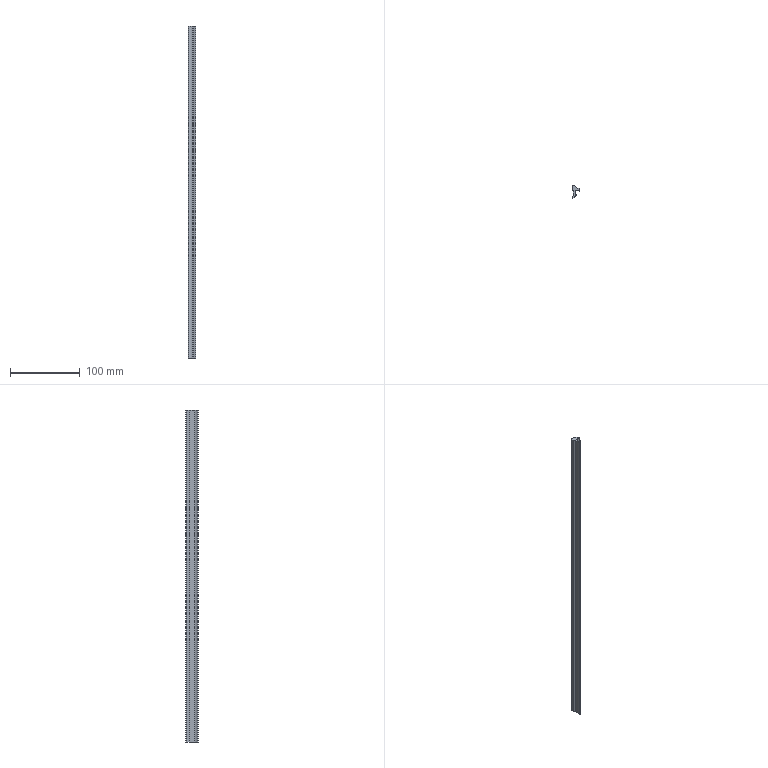Part | SolidWorks | features BaseBody 1, MoveFace 1 | 1 solid | 20 faces | box 10.8 x 17.5 x 476 mm | volume 37509 mm3 | cylinder 11 | plane 9 | commonest cylinder face diameters 1.6 x2 14 x2 0.4 x1 0.6 x1 0.8 x1 2.6 x1
STEP:
#1=CARTESIAN_POINT('',(-3.236,-11.055,376.));
#2=VERTEX_POINT('',#1);
#3=CARTESIAN_POINT('',(-4.3,-10.3,376.));
#4=VERTEX_POINT('',#3);
#5=CARTESIAN_POINT('',(-3.5,-10.3,376.));
#6=DIRECTION('',(0.,0.,-1.));
#7=DIRECTION('',(1.,0.,0.));
#8=AXIS2_PLACEMENT_3D('',#5,#6,#7);
#9=CIRCLE('',#8,0.8);
#10=EDGE_CURVE('',#2,#4,#9,.T.);
#11=ORIENTED_EDGE('',*,*,#10,.T.);
#12=CARTESIAN_POINT('',(-4.3,-10.3,-100.));
#13=VERTEX_POINT('',#12);
#14=CARTESIAN_POINT('',(-4.3,-10.3,-100.));
#15=DIRECTION('',(0.,0.,-1.));
#16=VECTOR('',#15,1000.);
#17=LINE('',#14,#16);
#18=EDGE_CURVE('',#4,#13,#17,.T.);
#19=ORIENTED_EDGE('',*,*,#18,.T.);
#20=CARTESIAN_POINT('',(-3.236,-11.055,-100.));
#21=VERTEX_POINT('',#20);
#22=CARTESIAN_POINT('',(-3.5,-10.3,-100.));
#23=DIRECTION('',(0.,0.,1.));
#24=DIRECTION('',(-1.,0.,0.));
#25=AXIS2_PLACEMENT_3D('',#22,#23,#24);
#26=CIRCLE('',#25,0.8);
#27=EDGE_CURVE('',#13,#21,#26,.T.);
#28=ORIENTED_EDGE('',*,*,#27,.T.);
#29=CARTESIAN_POINT('',(-3.236,-11.055,-100.));
#30=DIRECTION('',(0.,0.,-1.));
#31=VECTOR('',#30,1000.);
#32=LINE('',#29,#31);
#33=EDGE_CURVE('',#2,#21,#32,.T.);
#34=ORIENTED_EDGE('',*,*,#33,.F.);
#35=EDGE_LOOP('',(#11,#19,#28,#34));
#36=FACE_OUTER_BOUND('',#35,.T.);
#37=CARTESIAN_POINT('',(-3.5,-10.3,-100.));
#38=DIRECTION('',(0.,0.,-1.));
#39=DIRECTION('',(-1.,0.,0.));
#40=AXIS2_PLACEMENT_3D('',#37,#38,#39);
#41=CYLINDRICAL_SURFACE('',#40,0.8);
#42=ADVANCED_FACE('',(#36),#41,.T.);
#43=CARTESIAN_POINT('',(1.184,-6.397,-100.));
#44=VERTEX_POINT('',#43);
#45=CARTESIAN_POINT('',(-5.702,-4.29,-100.));
#46=DIRECTION('',(0.,0.,1.));
#47=DIRECTION('',(-1.,0.,0.));
#48=AXIS2_PLACEMENT_3D('',#45,#46,#47);
#49=CIRCLE('',#48,7.201);
#50=EDGE_CURVE('',#21,#44,#49,.T.);
#51=ORIENTED_EDGE('',*,*,#50,.T.);
#52=CARTESIAN_POINT('',(1.184,-6.397,376.));
#53=VERTEX_POINT('',#52);
#54=CARTESIAN_POINT('',(1.184,-6.397,-100.));
#55=DIRECTION('',(0.,0.,1.));
#56=VECTOR('',#55,1000.);
#57=LINE('',#54,#56);
#58=EDGE_CURVE('',#44,#53,#57,.T.);
#59=ORIENTED_EDGE('',*,*,#58,.T.);
#60=CARTESIAN_POINT('',(-5.702,-4.29,376.));
#61=DIRECTION('',(0.,0.,-1.));
#62=DIRECTION('',(1.,0.,0.));
#63=AXIS2_PLACEMENT_3D('',#60,#61,#62);
#64=CIRCLE('',#63,7.201);
#65=EDGE_CURVE('',#53,#2,#64,.T.);
#66=ORIENTED_EDGE('',*,*,#65,.T.);
#67=ORIENTED_EDGE('',*,*,#33,.T.);
#68=EDGE_LOOP('',(#51,#59,#66,#67));
#69=FACE_OUTER_BOUND('',#68,.T.);
#70=CARTESIAN_POINT('',(-5.702,-4.29,-100.));
#71=DIRECTION('',(0.,0.,-1.));
#72=DIRECTION('',(-1.,0.,0.));
#73=AXIS2_PLACEMENT_3D('',#70,#71,#72);
#74=CYLINDRICAL_SURFACE('',#73,7.201);
#75=ADVANCED_FACE('',(#69),#74,.T.);
#76=CARTESIAN_POINT('',(0.9,-6.,-100.));
#77=VERTEX_POINT('',#76);
#78=CARTESIAN_POINT('',(0.9,-6.3,-100.));
#79=DIRECTION('',(0.,0.,1.));
#80=DIRECTION('',(-1.,0.,0.));
#81=AXIS2_PLACEMENT_3D('',#78,#79,#80);
#82=CIRCLE('',#81,0.3);
#83=EDGE_CURVE('',#44,#77,#82,.T.);
#84=ORIENTED_EDGE('',*,*,#83,.T.);
#85=CARTESIAN_POINT('',(0.9,-6.,376.));
#86=VERTEX_POINT('',#85);
#87=CARTESIAN_POINT('',(0.9,-6.,-100.));
#88=DIRECTION('',(0.,0.,1.));
#89=VECTOR('',#88,1000.);
#90=LINE('',#87,#89);
#91=EDGE_CURVE('',#77,#86,#90,.T.);
#92=ORIENTED_EDGE('',*,*,#91,.T.);
#93=CARTESIAN_POINT('',(0.9,-6.3,376.));
#94=DIRECTION('',(0.,0.,-1.));
#95=DIRECTION('',(1.,0.,0.));
#96=AXIS2_PLACEMENT_3D('',#93,#94,#95);
#97=CIRCLE('',#96,0.3);
#98=EDGE_CURVE('',#86,#53,#97,.T.);
#99=ORIENTED_EDGE('',*,*,#98,.T.);
#100=ORIENTED_EDGE('',*,*,#58,.F.);
#101=EDGE_LOOP('',(#84,#92,#99,#100));
#102=FACE_OUTER_BOUND('',#101,.T.);
#103=CARTESIAN_POINT('',(0.9,-6.3,-100.));
#104=DIRECTION('',(0.,0.,-1.));
#105=DIRECTION('',(-1.,0.,0.));
#106=AXIS2_PLACEMENT_3D('',#103,#104,#105);
#107=CYLINDRICAL_SURFACE('',#106,0.3);
#108=ADVANCED_FACE('',(#102),#107,.T.);
#109=CARTESIAN_POINT('',(-2.5,-0.5,-100.));
#110=VERTEX_POINT('',#109);
#111=CARTESIAN_POINT('',(-2.5,-6.153,-100.));
#112=VERTEX_POINT('',#111);
#113=CARTESIAN_POINT('',(-2.5,-6.397,-100.));
#114=DIRECTION('',(0.,-1.,0.));
#115=VECTOR('',#114,1000.);
#116=LINE('',#113,#115);
#117=EDGE_CURVE('',#110,#112,#116,.T.);
#118=ORIENTED_EDGE('',*,*,#117,.F.);
#119=CARTESIAN_POINT('',(-4.2,1.695,-100.));
#120=VERTEX_POINT('',#119);
#121=CARTESIAN_POINT('',(-1.701,1.875,-100.));
#122=DIRECTION('',(0.,0.,1.));
#123=DIRECTION('',(-1.,0.,0.));
#124=AXIS2_PLACEMENT_3D('',#121,#122,#123);
#125=CIRCLE('',#124,2.506);
#126=EDGE_CURVE('',#120,#110,#125,.T.);
#127=ORIENTED_EDGE('',*,*,#126,.F.);
#128=CARTESIAN_POINT('',(-4.2,5.1,-100.));
#129=VERTEX_POINT('',#128);
#130=CARTESIAN_POINT('',(-4.2,-6.397,-100.));
#131=DIRECTION('',(0.,-1.,0.));
#132=VECTOR('',#131,1000.);
#133=LINE('',#130,#132);
#134=EDGE_CURVE('',#129,#120,#133,.T.);
#135=ORIENTED_EDGE('',*,*,#134,.F.);
#136=CARTESIAN_POINT('',(-2.892,6.4,-100.));
#137=VERTEX_POINT('',#136);
#138=CARTESIAN_POINT('',(-2.9,5.1,-100.));
#139=DIRECTION('',(0.,0.,1.));
#140=DIRECTION('',(-1.,0.,0.));
#141=AXIS2_PLACEMENT_3D('',#138,#139,#140);
#142=CIRCLE('',#141,1.3);
#143=EDGE_CURVE('',#137,#129,#142,.T.);
#144=ORIENTED_EDGE('',*,*,#143,.F.);
#145=CARTESIAN_POINT('',(0.5,5.5,-100.));
#146=VERTEX_POINT('',#145);
#147=CARTESIAN_POINT('',(-2.934,-0.5999,-100.));
#148=DIRECTION('',(0.,0.,1.));
#149=DIRECTION('',(-1.,0.,0.));
#150=AXIS2_PLACEMENT_3D('',#147,#148,#149);
#151=CIRCLE('',#150,7.);
#152=EDGE_CURVE('',#146,#137,#151,.T.);
#153=ORIENTED_EDGE('',*,*,#152,.F.);
#154=CARTESIAN_POINT('',(5.5,1.7,-100.));
#155=VERTEX_POINT('',#154);
#156=CARTESIAN_POINT('',(5.5,1.7,-100.));
#157=DIRECTION('',(-0.7962,0.6051,0.));
#158=VECTOR('',#157,1000.);
#159=LINE('',#156,#158);
#160=EDGE_CURVE('',#155,#146,#159,.T.);
#161=ORIENTED_EDGE('',*,*,#160,.F.);
#162=CARTESIAN_POINT('',(6.458,-0.2215,-100.));
#163=VERTEX_POINT('',#162);
#164=CARTESIAN_POINT('',(6.458,-0.2215,-100.));
#165=DIRECTION('',(-0.4462,0.8949,0.));
#166=VECTOR('',#165,1000.);
#167=LINE('',#164,#166);
#168=EDGE_CURVE('',#163,#155,#167,.T.);
#169=ORIENTED_EDGE('',*,*,#168,.F.);
#170=CARTESIAN_POINT('',(5.895,-0.7433,-100.));
#171=VERTEX_POINT('',#170);
#172=CARTESIAN_POINT('',(6.1,-0.4,-100.));
#173=DIRECTION('',(0.,0.,1.));
#174=DIRECTION('',(-1.,0.,0.));
#175=AXIS2_PLACEMENT_3D('',#172,#173,#174);
#176=CIRCLE('',#175,0.4);
#177=EDGE_CURVE('',#171,#163,#176,.T.);
#178=ORIENTED_EDGE('',*,*,#177,.F.);
#179=CARTESIAN_POINT('',(3.,0.,-100.));
#180=VERTEX_POINT('',#179);
#181=CARTESIAN_POINT('',(2.746,-6.995,-100.));
#182=DIRECTION('',(0.,0.,-1.));
#183=DIRECTION('',(-1.,0.,0.));
#184=AXIS2_PLACEMENT_3D('',#181,#182,#183);
#185=CIRCLE('',#184,7.);
#186=EDGE_CURVE('',#180,#171,#185,.T.);
#187=ORIENTED_EDGE('',*,*,#186,.F.);
#188=CARTESIAN_POINT('',(0.,0.,-100.));
#189=VERTEX_POINT('',#188);
#190=CARTESIAN_POINT('',(-6.814,0.,-100.));
#191=DIRECTION('',(1.,0.,0.));
#192=VECTOR('',#191,1000.);
#193=LINE('',#190,#192);
#194=EDGE_CURVE('',#189,#180,#193,.T.);
#195=ORIENTED_EDGE('',*,*,#194,.F.);
#196=CARTESIAN_POINT('',(0.,-5.8,-100.));
#197=VERTEX_POINT('',#196);
#198=CARTESIAN_POINT('',(0.,-6.397,-100.));
#199=DIRECTION('',(0.,1.,0.));
#200=VECTOR('',#199,1000.);
#201=LINE('',#198,#200);
#202=EDGE_CURVE('',#197,#189,#201,.T.);
#203=ORIENTED_EDGE('',*,*,#202,.F.);
#204=CARTESIAN_POINT('',(0.2,-6.,-100.));
#205=VERTEX_POINT('',#204);
#206=CARTESIAN_POINT('',(0.2,-5.8,-100.));
#207=DIRECTION('',(0.,0.,1.));
#208=DIRECTION('',(-1.,0.,0.));
#209=AXIS2_PLACEMENT_3D('',#206,#207,#208);
#210=CIRCLE('',#209,0.2);
#211=EDGE_CURVE('',#197,#205,#210,.T.);
#212=ORIENTED_EDGE('',*,*,#211,.T.);
#213=CARTESIAN_POINT('',(-6.814,-6.,-100.));
#214=DIRECTION('',(-1.,0.,0.));
#215=VECTOR('',#214,1000.);
#216=LINE('',#213,#215);
#217=EDGE_CURVE('',#77,#205,#216,.T.);
#218=ORIENTED_EDGE('',*,*,#217,.F.);
#219=ORIENTED_EDGE('',*,*,#83,.F.);
#220=ORIENTED_EDGE('',*,*,#50,.F.);
#221=ORIENTED_EDGE('',*,*,#27,.F.);
#222=CARTESIAN_POINT('',(-3.998,-9.674,-100.));
#223=VERTEX_POINT('',#222);
#224=CARTESIAN_POINT('',(-3.5,-10.3,-100.));
#225=DIRECTION('',(0.,0.,1.));
#226=DIRECTION('',(-1.,0.,0.));
#227=AXIS2_PLACEMENT_3D('',#224,#225,#226);
#228=CIRCLE('',#227,0.8);
#229=EDGE_CURVE('',#223,#13,#228,.T.);
#230=ORIENTED_EDGE('',*,*,#229,.F.);
#231=CARTESIAN_POINT('',(-6.814,-6.397,-100.));
#232=DIRECTION('',(0.,0.,-1.));
#233=DIRECTION('',(-1.,0.,0.));
#234=AXIS2_PLACEMENT_3D('',#231,#232,#233);
#235=CIRCLE('',#234,4.321);
#236=EDGE_CURVE('',#112,#223,#235,.T.);
#237=ORIENTED_EDGE('',*,*,#236,.F.);
#238=EDGE_LOOP('',(#118,#127,#135,#144,#153,#161,#169,#178,#187,#195,#203,#212,#218,#219,#220,#221,#230,#237));
#239=FACE_OUTER_BOUND('',#238,.T.);
#240=CARTESIAN_POINT('',(-6.814,-6.397,-100.));
#241=DIRECTION('',(0.,0.,1.));
#242=DIRECTION('',(1.,0.,0.));
#243=AXIS2_PLACEMENT_3D('',#240,#241,#242);
#244=PLANE('',#243);
#245=ADVANCED_FACE('',(#239),#244,.F.);
#246=ORIENTED_EDGE('',*,*,#18,.F.);
#247=CARTESIAN_POINT('',(-3.998,-9.674,376.));
#248=VERTEX_POINT('',#247);
#249=CARTESIAN_POINT('',(-3.5,-10.3,376.));
#250=DIRECTION('',(0.,0.,-1.));
#251=DIRECTION('',(1.,0.,0.));
#252=AXIS2_PLACEMENT_3D('',#249,#250,#251);
#253=CIRCLE('',#252,0.8);
#254=EDGE_CURVE('',#4,#248,#253,.T.);
#255=ORIENTED_EDGE('',*,*,#254,.T.);
#256=CARTESIAN_POINT('',(-3.998,-9.674,-100.));
#257=DIRECTION('',(0.,0.,-1.));
#258=VECTOR('',#257,1000.);
#259=LINE('',#256,#258);
#260=EDGE_CURVE('',#248,#223,#259,.T.);
#261=ORIENTED_EDGE('',*,*,#260,.T.);
#262=ORIENTED_EDGE('',*,*,#229,.T.);
#263=EDGE_LOOP('',(#246,#255,#261,#262));
#264=FACE_OUTER_BOUND('',#263,.T.);
#265=CARTESIAN_POINT('',(-3.5,-10.3,-100.));
#266=DIRECTION('',(0.,0.,-1.));
#267=DIRECTION('',(-1.,0.,0.));
#268=AXIS2_PLACEMENT_3D('',#265,#266,#267);
#269=CYLINDRICAL_SURFACE('',#268,0.8);
#270=ADVANCED_FACE('',(#264),#269,.T.);
#271=CARTESIAN_POINT('',(-4.2,1.695,376.));
#272=VERTEX_POINT('',#271);
#273=CARTESIAN_POINT('',(-2.5,-0.5,376.));
#274=VERTEX_POINT('',#273);
#275=CARTESIAN_POINT('',(-1.701,1.875,376.));
#276=DIRECTION('',(0.,0.,1.));
#277=DIRECTION('',(1.,0.,0.));
#278=AXIS2_PLACEMENT_3D('',#275,#276,#277);
#279=CIRCLE('',#278,2.506);
#280=EDGE_CURVE('',#272,#274,#279,.T.);
#281=ORIENTED_EDGE('',*,*,#280,.T.);
#282=CARTESIAN_POINT('',(-2.5,-6.153,376.));
#283=VERTEX_POINT('',#282);
#284=CARTESIAN_POINT('',(-2.5,-6.397,376.));
#285=DIRECTION('',(0.,-1.,0.));
#286=VECTOR('',#285,1000.);
#287=LINE('',#284,#286);
#288=EDGE_CURVE('',#274,#283,#287,.T.);
#289=ORIENTED_EDGE('',*,*,#288,.T.);
#290=CARTESIAN_POINT('',(-6.814,-6.397,376.));
#291=DIRECTION('',(0.,0.,-1.));
#292=DIRECTION('',(1.,0.,0.));
#293=AXIS2_PLACEMENT_3D('',#290,#291,#292);
#294=CIRCLE('',#293,4.321);
#295=EDGE_CURVE('',#283,#248,#294,.T.);
#296=ORIENTED_EDGE('',*,*,#295,.T.);
#297=ORIENTED_EDGE('',*,*,#254,.F.);
#298=ORIENTED_EDGE('',*,*,#10,.F.);
#299=ORIENTED_EDGE('',*,*,#65,.F.);
#300=ORIENTED_EDGE('',*,*,#98,.F.);
#301=CARTESIAN_POINT('',(0.2,-6.,376.));
#302=VERTEX_POINT('',#301);
#303=CARTESIAN_POINT('',(-6.814,-6.,376.));
#304=DIRECTION('',(-1.,0.,0.));
#305=VECTOR('',#304,1000.);
#306=LINE('',#303,#305);
#307=EDGE_CURVE('',#86,#302,#306,.T.);
#308=ORIENTED_EDGE('',*,*,#307,.T.);
#309=CARTESIAN_POINT('',(0.,-5.8,376.));
#310=VERTEX_POINT('',#309);
#311=CARTESIAN_POINT('',(0.2,-5.8,376.));
#312=DIRECTION('',(0.,0.,-1.));
#313=DIRECTION('',(1.,0.,0.));
#314=AXIS2_PLACEMENT_3D('',#311,#312,#313);
#315=CIRCLE('',#314,0.2);
#316=EDGE_CURVE('',#302,#310,#315,.T.);
#317=ORIENTED_EDGE('',*,*,#316,.T.);
#318=CARTESIAN_POINT('',(0.,0.,376.));
#319=VERTEX_POINT('',#318);
#320=CARTESIAN_POINT('',(0.,-6.397,376.));
#321=DIRECTION('',(0.,1.,0.));
#322=VECTOR('',#321,1000.);
#323=LINE('',#320,#322);
#324=EDGE_CURVE('',#310,#319,#323,.T.);
#325=ORIENTED_EDGE('',*,*,#324,.T.);
#326=CARTESIAN_POINT('',(3.,0.,376.));
#327=VERTEX_POINT('',#326);
#328=CARTESIAN_POINT('',(-6.814,0.,376.));
#329=DIRECTION('',(1.,0.,0.));
#330=VECTOR('',#329,1000.);
#331=LINE('',#328,#330);
#332=EDGE_CURVE('',#319,#327,#331,.T.);
#333=ORIENTED_EDGE('',*,*,#332,.T.);
#334=CARTESIAN_POINT('',(5.895,-0.7433,376.));
#335=VERTEX_POINT('',#334);
#336=CARTESIAN_POINT('',(2.746,-6.995,376.));
#337=DIRECTION('',(0.,0.,-1.));
#338=DIRECTION('',(1.,0.,0.));
#339=AXIS2_PLACEMENT_3D('',#336,#337,#338);
#340=CIRCLE('',#339,7.);
#341=EDGE_CURVE('',#327,#335,#340,.T.);
#342=ORIENTED_EDGE('',*,*,#341,.T.);
#343=CARTESIAN_POINT('',(6.458,-0.2215,376.));
#344=VERTEX_POINT('',#343);
#345=CARTESIAN_POINT('',(6.1,-0.4,376.));
#346=DIRECTION('',(0.,0.,-1.));
#347=DIRECTION('',(1.,0.,0.));
#348=AXIS2_PLACEMENT_3D('',#345,#346,#347);
#349=CIRCLE('',#348,0.4);
#350=EDGE_CURVE('',#344,#335,#349,.T.);
#351=ORIENTED_EDGE('',*,*,#350,.F.);
#352=CARTESIAN_POINT('',(5.5,1.7,376.));
#353=VERTEX_POINT('',#352);
#354=CARTESIAN_POINT('',(6.282,0.1323,376.));
#355=DIRECTION('',(-0.4462,0.8949,0.));
#356=VECTOR('',#355,1000.);
#357=LINE('',#354,#356);
#358=EDGE_CURVE('',#344,#353,#357,.T.);
#359=ORIENTED_EDGE('',*,*,#358,.T.);
#360=CARTESIAN_POINT('',(0.5,5.5,376.));
#361=VERTEX_POINT('',#360);
#362=CARTESIAN_POINT('',(1.595,4.668,376.));
#363=DIRECTION('',(-0.7962,0.6051,0.));
#364=VECTOR('',#363,1000.);
#365=LINE('',#362,#364);
#366=EDGE_CURVE('',#353,#361,#365,.T.);
#367=ORIENTED_EDGE('',*,*,#366,.T.);
#368=CARTESIAN_POINT('',(-2.892,6.4,376.));
#369=VERTEX_POINT('',#368);
#370=CARTESIAN_POINT('',(-2.934,-0.5999,376.));
#371=DIRECTION('',(0.,0.,1.));
#372=DIRECTION('',(1.,0.,0.));
#373=AXIS2_PLACEMENT_3D('',#370,#371,#372);
#374=CIRCLE('',#373,7.);
#375=EDGE_CURVE('',#361,#369,#374,.T.);
#376=ORIENTED_EDGE('',*,*,#375,.T.);
#377=CARTESIAN_POINT('',(-4.2,5.1,376.));
#378=VERTEX_POINT('',#377);
#379=CARTESIAN_POINT('',(-2.9,5.1,376.));
#380=DIRECTION('',(0.,0.,1.));
#381=DIRECTION('',(1.,0.,0.));
#382=AXIS2_PLACEMENT_3D('',#379,#380,#381);
#383=CIRCLE('',#382,1.3);
#384=EDGE_CURVE('',#369,#378,#383,.T.);
#385=ORIENTED_EDGE('',*,*,#384,.T.);
#386=CARTESIAN_POINT('',(-4.2,-6.397,376.));
#387=DIRECTION('',(0.,-1.,0.));
#388=VECTOR('',#387,1000.);
#389=LINE('',#386,#388);
#390=EDGE_CURVE('',#378,#272,#389,.T.);
#391=ORIENTED_EDGE('',*,*,#390,.T.);
#392=EDGE_LOOP('',(#281,#289,#296,#297,#298,#299,#300,#308,#317,#325,#333,#342,#351,#359,#367,#376,#385,#391));
#393=FACE_OUTER_BOUND('',#392,.T.);
#394=CARTESIAN_POINT('',(-6.814,-6.397,376.));
#395=DIRECTION('',(0.,0.,1.));
#396=DIRECTION('',(1.,0.,0.));
#397=AXIS2_PLACEMENT_3D('',#394,#395,#396);
#398=PLANE('',#397);
#399=ADVANCED_FACE('',(#393),#398,.T.);
#400=ORIENTED_EDGE('',*,*,#217,.T.);
#401=CARTESIAN_POINT('',(0.2,-6.,-100.));
#402=DIRECTION('',(0.,0.,1.));
#403=VECTOR('',#402,1000.);
#404=LINE('',#401,#403);
#405=EDGE_CURVE('',#205,#302,#404,.T.);
#406=ORIENTED_EDGE('',*,*,#405,.T.);
#407=ORIENTED_EDGE('',*,*,#307,.F.);
#408=ORIENTED_EDGE('',*,*,#91,.F.);
#409=EDGE_LOOP('',(#400,#406,#407,#408));
#410=FACE_OUTER_BOUND('',#409,.T.);
#411=CARTESIAN_POINT('',(0.9,-6.,-100.));
#412=DIRECTION('',(0.,1.,0.));
#413=DIRECTION('',(0.,0.,1.));
#414=AXIS2_PLACEMENT_3D('',#411,#412,#413);
#415=PLANE('',#414);
#416=ADVANCED_FACE('',(#410),#415,.T.);
#417=CARTESIAN_POINT('',(-2.5,-6.153,-100.));
#418=DIRECTION('',(0.,0.,1.));
#419=VECTOR('',#418,1000.);
#420=LINE('',#417,#419);
#421=EDGE_CURVE('',#112,#283,#420,.T.);
#422=ORIENTED_EDGE('',*,*,#421,.F.);
#423=ORIENTED_EDGE('',*,*,#236,.T.);
#424=ORIENTED_EDGE('',*,*,#260,.F.);
#425=ORIENTED_EDGE('',*,*,#295,.F.);
#426=EDGE_LOOP('',(#422,#423,#424,#425));
#427=FACE_OUTER_BOUND('',#426,.T.);
#428=CARTESIAN_POINT('',(-6.814,-6.397,-100.));
#429=DIRECTION('',(0.,0.,-1.));
#430=DIRECTION('',(-1.,0.,0.));
#431=AXIS2_PLACEMENT_3D('',#428,#429,#430);
#432=CYLINDRICAL_SURFACE('',#431,4.321);
#433=ADVANCED_FACE('',(#427),#432,.F.);
#434=ORIENTED_EDGE('',*,*,#117,.T.);
#435=ORIENTED_EDGE('',*,*,#421,.T.);
#436=ORIENTED_EDGE('',*,*,#288,.F.);
#437=CARTESIAN_POINT('',(-2.5,-0.5,-100.));
#438=DIRECTION('',(0.,0.,-1.));
#439=VECTOR('',#438,1000.);
#440=LINE('',#437,#439);
#441=EDGE_CURVE('',#274,#110,#440,.T.);
#442=ORIENTED_EDGE('',*,*,#441,.T.);
#443=EDGE_LOOP('',(#434,#435,#436,#442));
#444=FACE_OUTER_BOUND('',#443,.T.);
#445=CARTESIAN_POINT('',(-2.5,-0.5,-100.));
#446=DIRECTION('',(-1.,0.,0.));
#447=DIRECTION('',(0.,0.,1.));
#448=AXIS2_PLACEMENT_3D('',#445,#446,#447);
#449=PLANE('',#448);
#450=ADVANCED_FACE('',(#444),#449,.T.);
#451=ORIENTED_EDGE('',*,*,#126,.T.);
#452=ORIENTED_EDGE('',*,*,#441,.F.);
#453=ORIENTED_EDGE('',*,*,#280,.F.);
#454=CARTESIAN_POINT('',(-4.2,1.695,-100.));
#455=DIRECTION('',(0.,0.,-1.));
#456=VECTOR('',#455,1000.);
#457=LINE('',#454,#456);
#458=EDGE_CURVE('',#272,#120,#457,.T.);
#459=ORIENTED_EDGE('',*,*,#458,.T.);
#460=EDGE_LOOP('',(#451,#452,#453,#459));
#461=FACE_OUTER_BOUND('',#460,.T.);
#462=CARTESIAN_POINT('',(-1.701,1.875,-100.));
#463=DIRECTION('',(0.,0.,-1.));
#464=DIRECTION('',(-1.,0.,0.));
#465=AXIS2_PLACEMENT_3D('',#462,#463,#464);
#466=CYLINDRICAL_SURFACE('',#465,2.506);
#467=ADVANCED_FACE('',(#461),#466,.T.);
#468=ORIENTED_EDGE('',*,*,#134,.T.);
#469=ORIENTED_EDGE('',*,*,#458,.F.);
#470=ORIENTED_EDGE('',*,*,#390,.F.);
#471=CARTESIAN_POINT('',(-4.2,5.1,-100.));
#472=DIRECTION('',(0.,0.,-1.));
#473=VECTOR('',#472,1000.);
#474=LINE('',#471,#473);
#475=EDGE_CURVE('',#378,#129,#474,.T.);
#476=ORIENTED_EDGE('',*,*,#475,.T.);
#477=EDGE_LOOP('',(#468,#469,#470,#476));
#478=FACE_OUTER_BOUND('',#477,.T.);
#479=CARTESIAN_POINT('',(-4.2,5.1,-100.));
#480=DIRECTION('',(-1.,0.,0.));
#481=DIRECTION('',(0.,0.,1.));
#482=AXIS2_PLACEMENT_3D('',#479,#480,#481);
#483=PLANE('',#482);
#484=ADVANCED_FACE('',(#478),#483,.T.);
#485=ORIENTED_EDGE('',*,*,#143,.T.);
#486=ORIENTED_EDGE('',*,*,#475,.F.);
#487=ORIENTED_EDGE('',*,*,#384,.F.);
#488=CARTESIAN_POINT('',(-2.892,6.4,-100.));
#489=DIRECTION('',(0.,0.,-1.));
#490=VECTOR('',#489,1000.);
#491=LINE('',#488,#490);
#492=EDGE_CURVE('',#369,#137,#491,.T.);
#493=ORIENTED_EDGE('',*,*,#492,.T.);
#494=EDGE_LOOP('',(#485,#486,#487,#493));
#495=FACE_OUTER_BOUND('',#494,.T.);
#496=CARTESIAN_POINT('',(-2.9,5.1,-100.));
#497=DIRECTION('',(0.,0.,-1.));
#498=DIRECTION('',(-1.,0.,0.));
#499=AXIS2_PLACEMENT_3D('',#496,#497,#498);
#500=CYLINDRICAL_SURFACE('',#499,1.3);
#501=ADVANCED_FACE('',(#495),#500,.T.);
#502=ORIENTED_EDGE('',*,*,#152,.T.);
#503=ORIENTED_EDGE('',*,*,#492,.F.);
#504=ORIENTED_EDGE('',*,*,#375,.F.);
#505=CARTESIAN_POINT('',(0.5,5.5,-100.));
#506=DIRECTION('',(0.,0.,-1.));
#507=VECTOR('',#506,1000.);
#508=LINE('',#505,#507);
#509=EDGE_CURVE('',#361,#146,#508,.T.);
#510=ORIENTED_EDGE('',*,*,#509,.T.);
#511=EDGE_LOOP('',(#502,#503,#504,#510));
#512=FACE_OUTER_BOUND('',#511,.T.);
#513=CARTESIAN_POINT('',(-2.934,-0.5999,-100.));
#514=DIRECTION('',(0.,0.,-1.));
#515=DIRECTION('',(-1.,0.,0.));
#516=AXIS2_PLACEMENT_3D('',#513,#514,#515);
#517=CYLINDRICAL_SURFACE('',#516,7.);
#518=ADVANCED_FACE('',(#512),#517,.T.);
#519=ORIENTED_EDGE('',*,*,#160,.T.);
#520=ORIENTED_EDGE('',*,*,#509,.F.);
#521=ORIENTED_EDGE('',*,*,#366,.F.);
#522=CARTESIAN_POINT('',(5.5,1.7,-100.));
#523=DIRECTION('',(0.,0.,-1.));
#524=VECTOR('',#523,1000.);
#525=LINE('',#522,#524);
#526=EDGE_CURVE('',#353,#155,#525,.T.);
#527=ORIENTED_EDGE('',*,*,#526,.T.);
#528=EDGE_LOOP('',(#519,#520,#521,#527));
#529=FACE_OUTER_BOUND('',#528,.T.);
#530=CARTESIAN_POINT('',(5.5,1.7,-100.));
#531=DIRECTION('',(0.6051,0.7962,0.));
#532=DIRECTION('',(-0.7962,0.6051,0.));
#533=AXIS2_PLACEMENT_3D('',#530,#531,#532);
#534=PLANE('',#533);
#535=ADVANCED_FACE('',(#529),#534,.T.);
#536=ORIENTED_EDGE('',*,*,#168,.T.);
#537=ORIENTED_EDGE('',*,*,#526,.F.);
#538=ORIENTED_EDGE('',*,*,#358,.F.);
#539=CARTESIAN_POINT('',(6.458,-0.2215,-100.));
#540=DIRECTION('',(0.,0.,-1.));
#541=VECTOR('',#540,1000.);
#542=LINE('',#539,#541);
#543=EDGE_CURVE('',#344,#163,#542,.T.);
#544=ORIENTED_EDGE('',*,*,#543,.T.);
#545=EDGE_LOOP('',(#536,#537,#538,#544));
#546=FACE_OUTER_BOUND('',#545,.T.);
#547=CARTESIAN_POINT('',(6.458,-0.2215,-100.));
#548=DIRECTION('',(0.8949,0.4462,0.));
#549=DIRECTION('',(-0.4462,0.8949,0.));
#550=AXIS2_PLACEMENT_3D('',#547,#548,#549);
#551=PLANE('',#550);
#552=ADVANCED_FACE('',(#546),#551,.T.);
#553=CARTESIAN_POINT('',(3.,0.,-100.));
#554=DIRECTION('',(0.,0.,1.));
#555=VECTOR('',#554,1000.);
#556=LINE('',#553,#555);
#557=EDGE_CURVE('',#180,#327,#556,.T.);
#558=ORIENTED_EDGE('',*,*,#557,.F.);
#559=ORIENTED_EDGE('',*,*,#186,.T.);
#560=CARTESIAN_POINT('',(5.895,-0.7433,-100.));
#561=DIRECTION('',(0.,0.,-1.));
#562=VECTOR('',#561,1000.);
#563=LINE('',#560,#562);
#564=EDGE_CURVE('',#335,#171,#563,.T.);
#565=ORIENTED_EDGE('',*,*,#564,.F.);
#566=ORIENTED_EDGE('',*,*,#341,.F.);
#567=EDGE_LOOP('',(#558,#559,#565,#566));
#568=FACE_OUTER_BOUND('',#567,.T.);
#569=CARTESIAN_POINT('',(2.746,-6.995,-100.));
#570=DIRECTION('',(0.,0.,-1.));
#571=DIRECTION('',(-1.,0.,0.));
#572=AXIS2_PLACEMENT_3D('',#569,#570,#571);
#573=CYLINDRICAL_SURFACE('',#572,7.);
#574=ADVANCED_FACE('',(#568),#573,.F.);
#575=ORIENTED_EDGE('',*,*,#194,.T.);
#576=ORIENTED_EDGE('',*,*,#557,.T.);
#577=ORIENTED_EDGE('',*,*,#332,.F.);
#578=CARTESIAN_POINT('',(0.,0.,-100.));
#579=DIRECTION('',(0.,0.,-1.));
#580=VECTOR('',#579,1000.);
#581=LINE('',#578,#580);
#582=EDGE_CURVE('',#319,#189,#581,.T.);
#583=ORIENTED_EDGE('',*,*,#582,.T.);
#584=EDGE_LOOP('',(#575,#576,#577,#583));
#585=FACE_OUTER_BOUND('',#584,.T.);
#586=CARTESIAN_POINT('',(0.,0.,-100.));
#587=DIRECTION('',(0.,-1.,0.));
#588=DIRECTION('',(0.,0.,-1.));
#589=AXIS2_PLACEMENT_3D('',#586,#587,#588);
#590=PLANE('',#589);
#591=ADVANCED_FACE('',(#585),#590,.T.);
#592=ORIENTED_EDGE('',*,*,#202,.T.);
#593=ORIENTED_EDGE('',*,*,#582,.F.);
#594=ORIENTED_EDGE('',*,*,#324,.F.);
#595=CARTESIAN_POINT('',(0.,-5.8,-100.));
#596=DIRECTION('',(0.,0.,-1.));
#597=VECTOR('',#596,1000.);
#598=LINE('',#595,#597);
#599=EDGE_CURVE('',#310,#197,#598,.T.);
#600=ORIENTED_EDGE('',*,*,#599,.T.);
#601=EDGE_LOOP('',(#592,#593,#594,#600));
#602=FACE_OUTER_BOUND('',#601,.T.);
#603=CARTESIAN_POINT('',(0.,-5.8,-100.));
#604=DIRECTION('',(1.,0.,0.));
#605=DIRECTION('',(0.,0.,-1.));
#606=AXIS2_PLACEMENT_3D('',#603,#604,#605);
#607=PLANE('',#606);
#608=ADVANCED_FACE('',(#602),#607,.T.);
#609=ORIENTED_EDGE('',*,*,#405,.F.);
#610=ORIENTED_EDGE('',*,*,#211,.F.);
#611=ORIENTED_EDGE('',*,*,#599,.F.);
#612=ORIENTED_EDGE('',*,*,#316,.F.);
#613=EDGE_LOOP('',(#609,#610,#611,#612));
#614=FACE_OUTER_BOUND('',#613,.T.);
#615=CARTESIAN_POINT('',(0.2,-5.8,-100.));
#616=DIRECTION('',(0.,0.,-1.));
#617=DIRECTION('',(-1.,0.,0.));
#618=AXIS2_PLACEMENT_3D('',#615,#616,#617);
#619=CYLINDRICAL_SURFACE('',#618,0.2);
#620=ADVANCED_FACE('',(#614),#619,.F.);
#621=ORIENTED_EDGE('',*,*,#177,.T.);
#622=ORIENTED_EDGE('',*,*,#543,.F.);
#623=ORIENTED_EDGE('',*,*,#350,.T.);
#624=ORIENTED_EDGE('',*,*,#564,.T.);
#625=EDGE_LOOP('',(#621,#622,#623,#624));
#626=FACE_OUTER_BOUND('',#625,.T.);
#627=CARTESIAN_POINT('',(6.1,-0.4,-100.));
#628=DIRECTION('',(0.,0.,-1.));
#629=DIRECTION('',(-1.,0.,0.));
#630=AXIS2_PLACEMENT_3D('',#627,#628,#629);
#631=CYLINDRICAL_SURFACE('',#630,0.4);
#632=ADVANCED_FACE('',(#626),#631,.T.);
#633=CLOSED_SHELL('',(#42,#75,#108,#245,#270,#399,#416,#433,#450,#467,#484,#501,#518,#535,#552,#574,#591,#608,#620,#632));
#634=MANIFOLD_SOLID_BREP('',#633);
#635=CARTESIAN_POINT('',(0.,0.,0.));
#636=DIRECTION('',(0.,0.,1.));
#637=DIRECTION('',(1.,0.,0.));
#638=AXIS2_PLACEMENT_3D('',#635,#636,#637);
#639=(LENGTH_UNIT()NAMED_UNIT(*)SI_UNIT(.MILLI.,.METRE.));
#640=UNCERTAINTY_MEASURE_WITH_UNIT(LENGTH_MEASURE(0.00001),#639,'','');
#641=(NAMED_UNIT(*)PLANE_ANGLE_UNIT()SI_UNIT($,.RADIAN.));
#642=(NAMED_UNIT(*)SI_UNIT($,.STERADIAN.)SOLID_ANGLE_UNIT());
#643=(GEOMETRIC_REPRESENTATION_CONTEXT(3)GLOBAL_UNCERTAINTY_ASSIGNED_CONTEXT((#640))GLOBAL_UNIT_ASSIGNED_CONTEXT((#639,#641,#642))REPRESENTATION_CONTEXT('',''));
#644=ADVANCED_BREP_SHAPE_REPRESENTATION('',(#634,#638),#643);